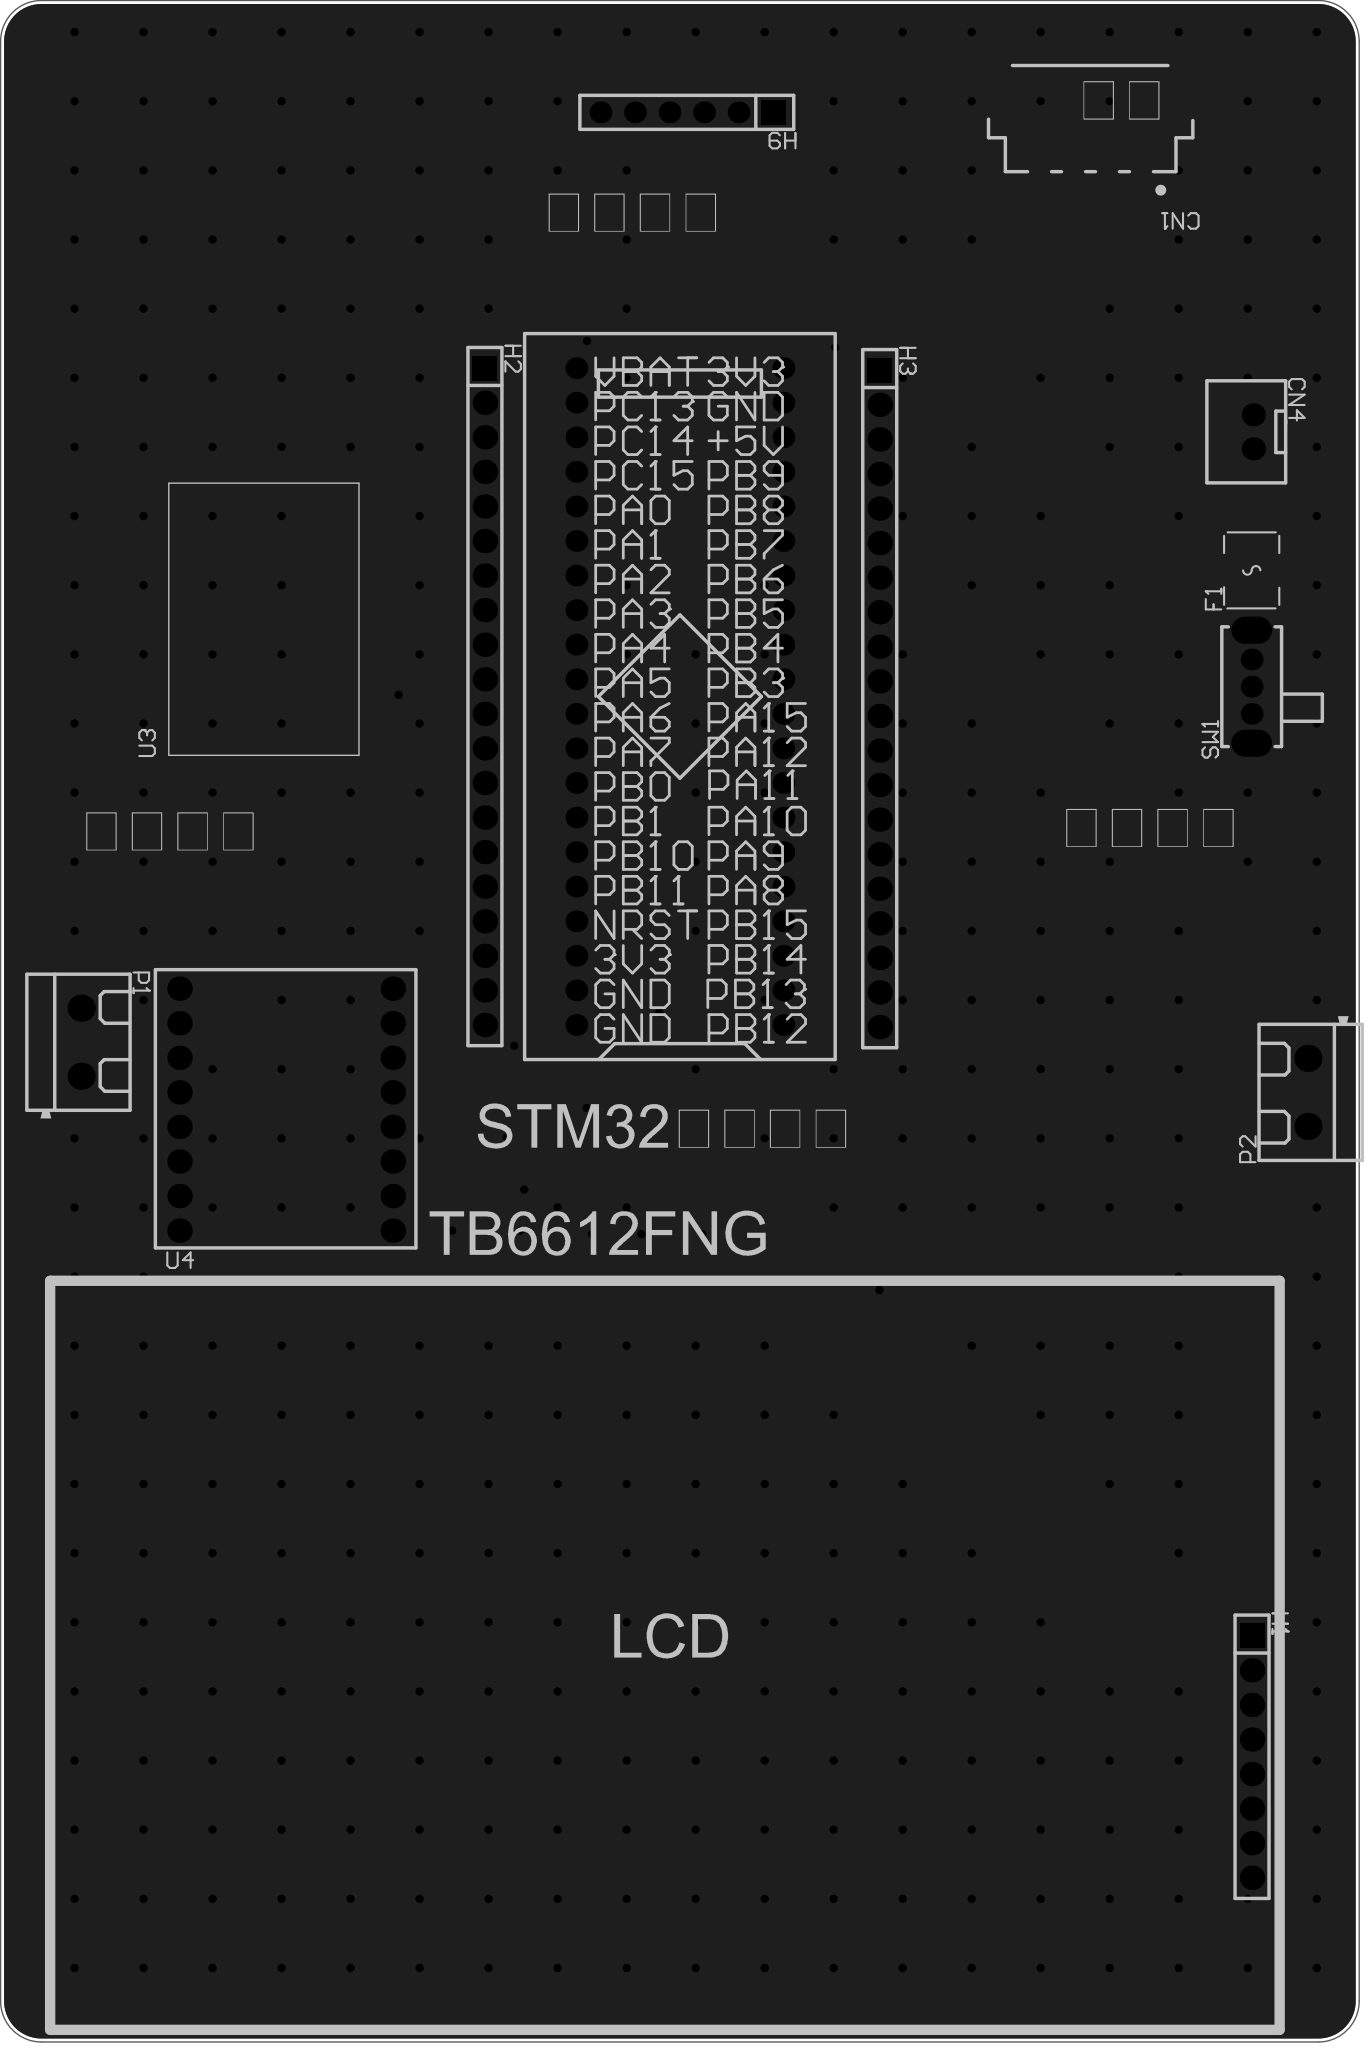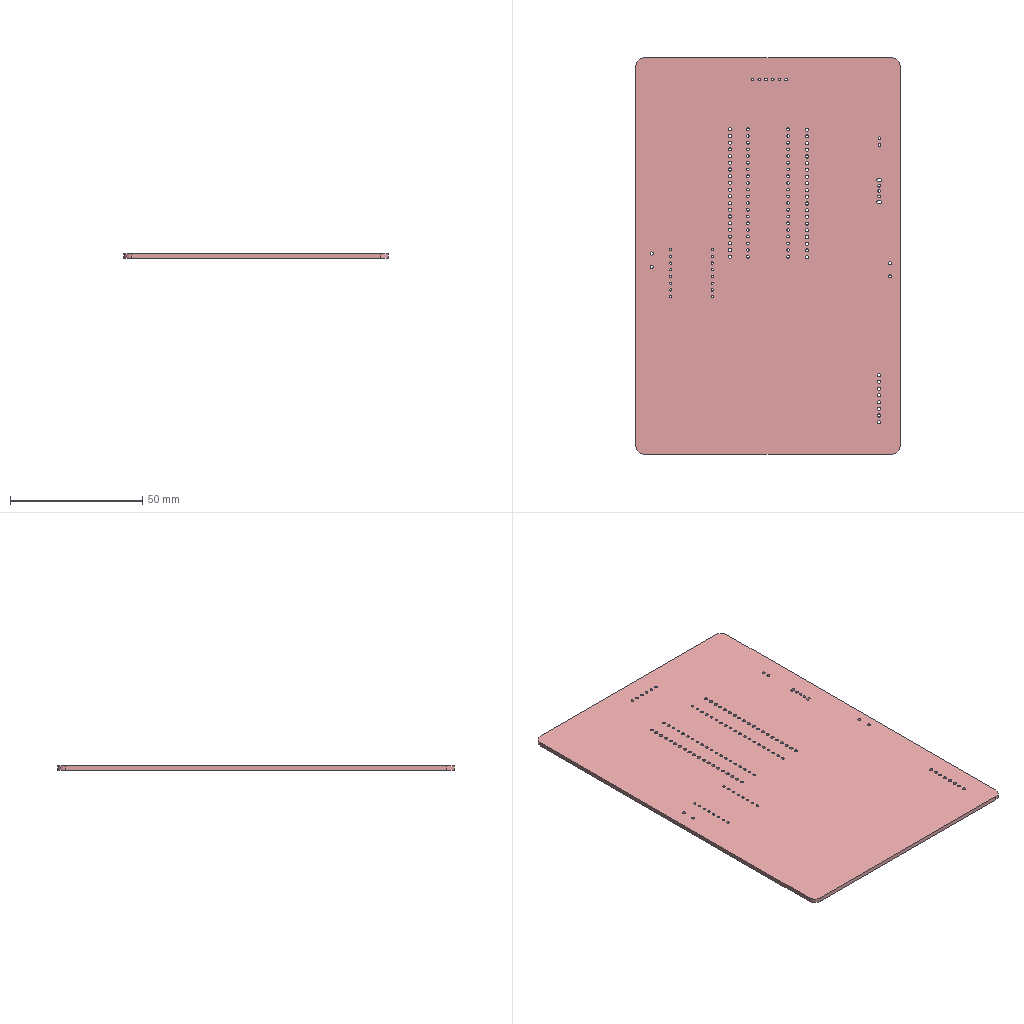Circuit board layout | Altium Designer | box 100 x 150 x 1.6 mm
Layer stack:
# Altium Designer layer stack of  (unit mm; dielectric type: 0 none, 1 core, 2 prepreg, 3 surface material)
index,name,kind,layer,copper_thickness_mm,dielectric_type,dielectric_thickness_mm,dielectric_material,dielectric_constant
0,Top Paste Mask Layer,other,,,,,,
1,Top Silkscreen Layer,other,,,,,,
2,Top Solder Mask Layer,dielectric,,,3,0.01,,3.3
3,Top Layer,copper,Top Layer,0.035,,,,
4,Dielectric1,dielectric,,,3,1.51,FR4,4.5
5,Bottom Layer,copper,Bottom Layer,0.035,,,,
6,Bottom Solder Mask Layer,dielectric,,,3,0.01,,3.3
7,Bottom Silkscreen Layer,other,,,,,,
8,Bottom Paste Mask Layer,other,,,,,,
# drill layer pairs: low layer,high layer
drill_pair,Top Layer,Bottom Layer
Part placement:
Designator,Comment,Layer,Footprint,Center-X(mm),Center-Y(mm),Rotation
U1,STM32F103C8T6-Card,TopLayer,CONN-TH_L53.3-W22.9_STM32F103C8T6-CARD,212.555,312.166,90
CN4,XH2.54*2P_直插,TopLayer,CONN-TH_2P-P2.50-XH2.54-2P,254.77,331.618,270
H9,,TopLayer,HDR-TH_6P-P2.54-V-F,213.063,355.092,180
U3,,TopLayer,EWM22M-400/900T22S,181.933,318.348,90
U4,,TopLayer,tb6612,183.574,281.813,0
CN1,XH2.54-4P,TopLayer,CONN-SMD_4P-P2.50-WT,242.781,353.314,180
P1,KF301-2P接线端子,TopLayer,CONN-TH_XY301V-A-5.0-2P,168.486,286.766,270
P2,KF301-2P接线端子,TopLayer,CONN-TH_XY301V-A-5.0-2P,258.783,283.083,90
F1,SMD1812-300-24,TopLayer,F1812,254.643,321.438,90
H1,,TopLayer,HDR-TH_8P-P2.54-V-F-1,254.668,234.266,270
SW1,,TopLayer,拨动开关_侧,254.643,312.892,90
H2,,TopLayer,HDR-TH_20P-P2.54-V-F,198.204,312.166,270
H3,,TopLayer,HDR-TH_20P-P2.54-V-F,227.264,312.012,270
Pad and via stacks:
# Altium Designer via and pad stacks of  (unit mm). Each distinct definition once, with the count of objects using it.
# via: kind,start_layer,end_layer,hole_mm,diameter_mm,mode(0 simple;1 top-mid-bottom;2 full stack),diameter_per_layer,count,example_net
# pad: kind,layer,hole_mm,hole_type(0 round;1 square;2 slot),plating,top_size,top_shape(1 round;2 rect;3 octagon;9 rounded rect),mid_size,bottom_size,mode,footprint,size_per_layer,count,example
pad,Multi-Layer,1,0,plated,1.6x1.6,1,1.6x1.6,1.6x1.6,0,CONN-TH_L53.3-W22.9_STM32F103C8T6-CARD,,40,U1.1
pad,Multi-Layer,1.05,0,plated,1.7x1.7,1,1.7x1.7,1.7x1.7,0,CONN-TH_2P-P2.50-XH2.54-2P,,2,CN4.2
pad,Multi-Layer,1.02,0,plated,1.6x1.6,1,1.6x1.6,1.6x1.6,0,HDR-TH_6P-P2.54-V-F,,5,H9.6
pad,Multi-Layer,1.02,0,plated,1.8x1.8,2,1.8x1.8,1.8x1.8,0,HDR-TH_6P-P2.54-V-F,,1,H9.1
pad,Multi-Layer,0.9,0,plated,1.8x1.8,1,1.8x1.8,1.8x1.8,0,tb6612,,16,U4.1
pad,Multi-Layer,1.2,0,plated,2x2,1,2x2,2x2,0,CONN-TH_XY301V-A-5.0-2P,,4,P1.1
pad,Multi-Layer,1.2,0,plated,1.8x1.8,2,1.8x1.8,1.8x1.8,0,HDR-TH_8P-P2.54-V-F-1,,1,H1.1
pad,Multi-Layer,1.2,0,plated,1.8x1.8,1,1.8x1.8,1.8x1.8,0,HDR-TH_8P-P2.54-V-F-1,,7,H1.2
pad,Multi-Layer,1.001,0,plated,1.6x1.6,1,1.6x1.6,1.6x1.6,0,\u00B2\u00A6\u00B6\u00AF\u00BF\u00AA\u00B9\u00D8_\u00B2\u00E0,,3,SW1.1
pad,Multi-Layer,1.001,2,plated,3x1.999,1,3x1.999,3x1.999,0,\u00B2\u00A6\u00B6\u00AF\u00BF\u00AA\u00B9\u00D8_\u00B2\u00E0,,2,SW1.4
pad,Multi-Layer,1.2,0,plated,1.8x1.8,2,1.8x1.8,1.8x1.8,0,HDR-TH_20P-P2.54-V-F,,2,H2.1
pad,Multi-Layer,1.2,0,plated,1.8x1.8,1,1.8x1.8,1.8x1.8,0,HDR-TH_20P-P2.54-V-F,,38,H2.2
pad,Top Layer,0,0,plated,0.85x1.8,2,0.85x1.8,0.85x1.8,0,EWM22M-400/900T22S,,24,U3.1
pad,Top Layer,0,0,plated,1.3x4,2,1.3x4,1.3x4,0,CONN-SMD_4P-P2.50-WT,,4,CN1.1
pad,Top Layer,0,0,plated,1.9x4,2,1.9x4,1.9x4,0,CONN-SMD_4P-P2.50-WT,,2,CN1.5
pad,Top Layer,0,0,plated,1.407x3.499,2,1.407x3.499,1.407x3.499,0,F1812,,2,F1.2
via,Top Layer,Bottom Layer,0.3048,0.61,0,,421,PB12
Copper pours:
name,layer,net,type(0 solid;1 hatched;2 none)
Top Layer-GND,Top Layer,GND,0
Bottom Layer-GND,Bottom Layer,GND,0
Design rules, without the lines most boards share:
# Altium Designer design rules of  (exported by Altium Designer, unit mm)
# columns: name | kind | enabled | priority | scope1 | scope2 | descriptor | typed fields (field=value)
Copper_copperRegion_copperThickness1oz | 0 | disabled | 4 | All | All | Clearance Constraint (Gap=5.984mil) (Disabled)(All),(All) | gap=0.152
Copper_copperRegion_copperThickness1oz_1 | 63 | disabled | 4 | All | All | Board Clearance Constraint (Gap=0mil) (Disabled)(All) |
Copper_copperRegion_Copper_copperRegion | 0 | disabled | 5 | All | All | Clearance Constraint (Gap=5.984mil) (Disabled)(All),(All) | gap=0.152
Copper_copperRegion_Copper_copperRegion_1 | 63 | disabled | 5 | All | All | Board Clearance Constraint (Gap=0mil) (Disabled)(All) |
copperThickness1oz | 0 | enabled | 6 | All | All | Clearance Constraint (Gap=5.984mil) (All),(All) | gap=0.152
copperThickness1oz_1 | 63 | enabled | 6 | All | All | Board Clearance Constraint (Gap=0mil) (All) |
copperThickness1oz_2 | 2 | enabled | 2 | All | All | Width Constraint (Min=30mil) (Max=100mil) (Preferred=30mil) (All) |
copperRegion_copperThickness1oz | 20 | disabled | 1 | All | All | Polygon Connect Rule(Relief Connect )(Conductor Width=10mil) (Relief Angle=90 Angle) (Entries=4) (Air Gap Width=10mil) (Disabled)(All),(All) | connect_style(0=relief,1=direct,2=none)=0 relief_conductor_width=0.254 relief_entries=4
copperRegion_Copper_copperRegion | 20 | disabled | 2 | All | All | Polygon Connect Rule(Relief Connect )(Conductor Width=10mil) (Relief Angle=90 Angle) (Entries=4) (Air Gap Width=10mil) (Disabled)(All),(All) | connect_style(0=relief,1=direct,2=none)=0 relief_conductor_width=0.254 relief_entries=4
copperRegion | 20 | enabled | 3 | All | All | Polygon Connect Rule(Relief Connect )(Conductor Width=10mil) (Relief Angle=90 Angle) (Entries=4) (Air Gap Width=10mil) (All),(All) | connect_style(0=relief,1=direct,2=none)=0 relief_conductor_width=0.254 relief_entries=4